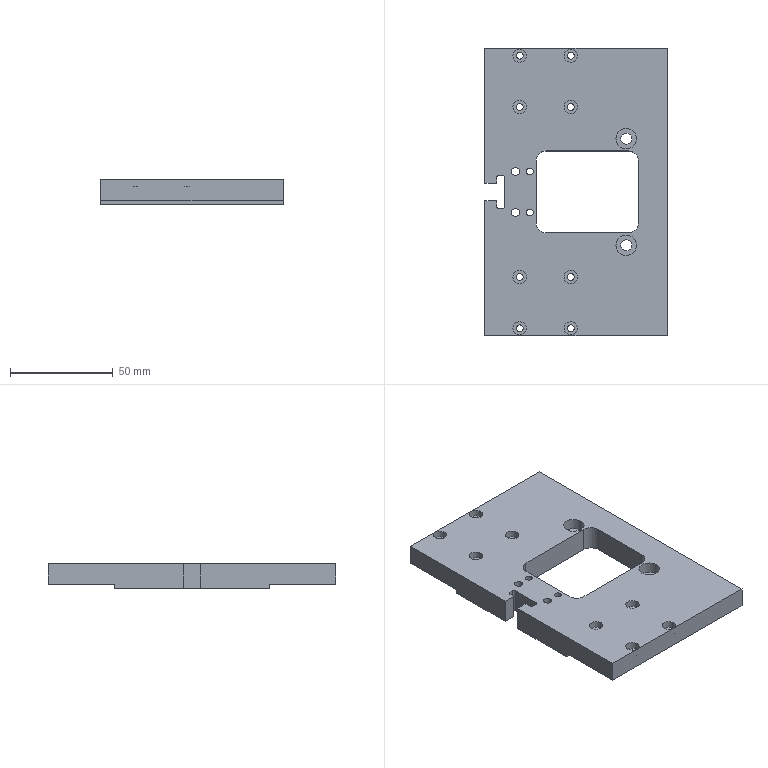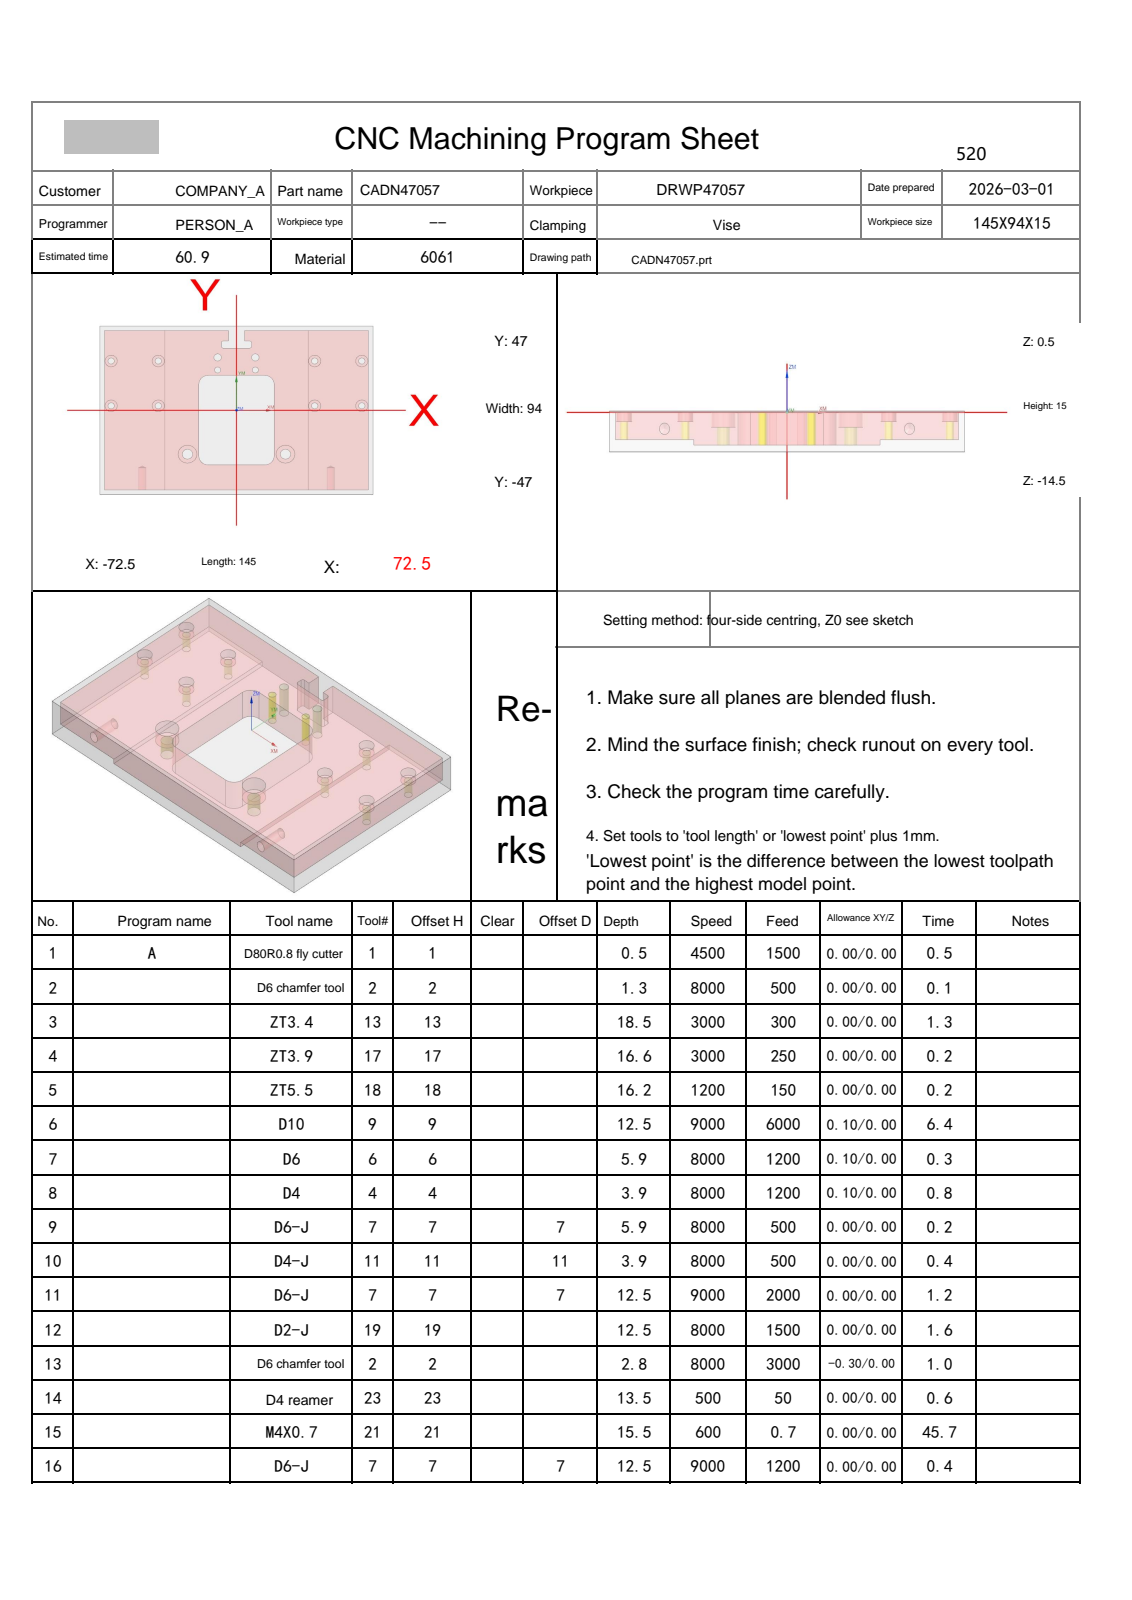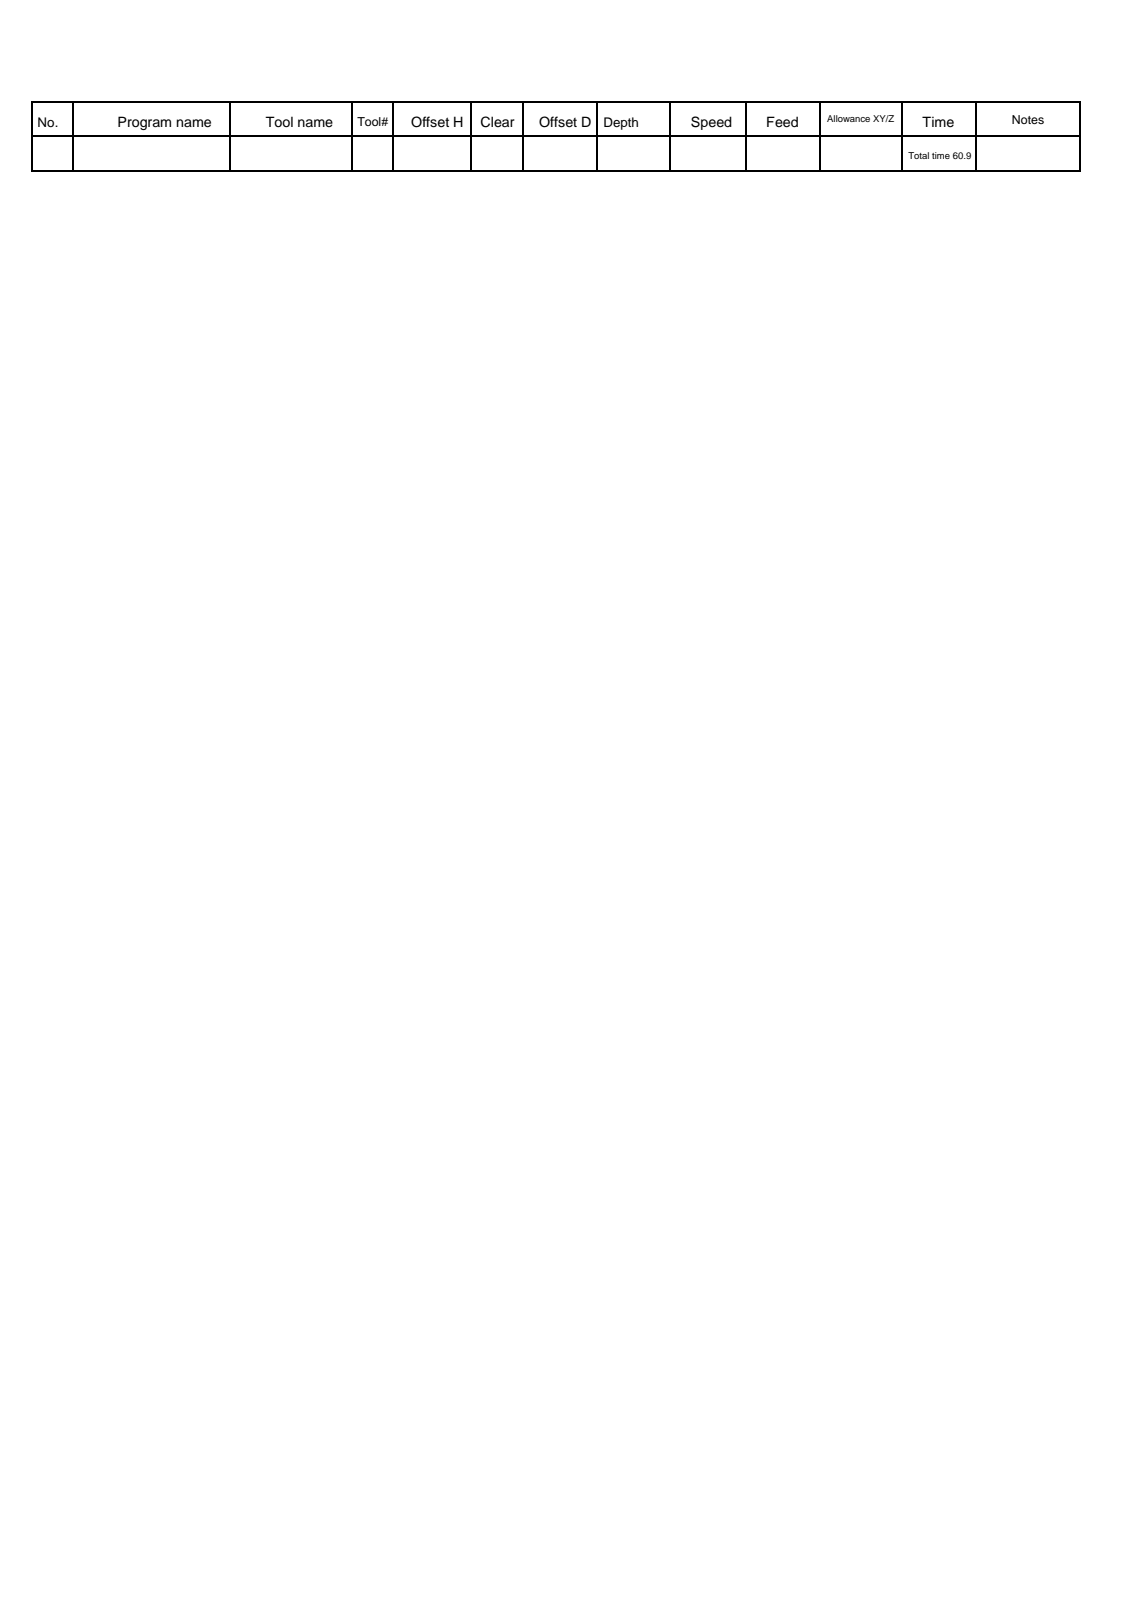NC program | NX | posted by the shop | part box 89 x 140 x 12 mm
Lines 949 to 2683 of 6684, first 1392 of 1735 lines:
N11 T07 M06
(D6-J  D=6. R=0. H=07 ce=0.00 di=0.00)
G00 G90 G54 X16.75 Y-5.7 M03 S9000
G43 H07 Z50.
M08
Z-5.45
G01 Z-5.95 F600.
G41 D07
X16.8
G03 X17. Y-5.5 I0.0 J.2
G01 Y14.5
G03 X15. Y16.5 I-2. J0.0
G01 X-15.
G03 X-17. Y14.5 I0.0 J-2.
G01 Y-25.5
G03 X-15. Y-27.5 I2. J0.0
G01 X15.
G03 X17. Y-25.5 I0.0 J2.
G01 Y-5.5
Y-5.
G03 X16.8 Y-4.8 I-.2 J0.0
G01 G40 X16.75
Z-5.45
G00 Z1.
Y-5.7
Z-11.4
G01 Z-11.9
G41 D07
X16.8
G03 X17. Y-5.5 I0.0 J.2
G01 Y14.5
G03 X15. Y16.5 I-2. J0.0
G01 X-15.
G03 X-17. Y14.5 I0.0 J-2.
G01 Y-25.5
G03 X-15. Y-27.5 I2. J0.0
G01 X15.
G03 X17. Y-25.5 I0.0 J2.
G01 Y-5.5
Y-5.
G03 X16.8 Y-4.8 I-.2 J0.0
G01 G40 X16.75
Z-11.4
G00 Z50.
G00 G90 X-2.228 Y47.539 M03 S8000
Z50.
Z.35
G01 X-2.232 Y47.532 Z.259 F2000.
X-2.243 Y47.513 Z.177
X-2.259 Y47.482 Z.103
X-2.278 Y47.441 Z.038
X-2.299 Y47.392 Z-.019
X-2.319 Y47.335 Z-.069
X-2.338 Y47.271 Z-.111
X-2.352 Y47.203 Z-.147
X-2.362 Y47.131 Z-.177
X-2.363 Y47.056 Z-.201
X-2.356 Y46.98 Z-.22
X-2.338 Y46.905 Z-.234
X-2.307 Y46.83 Z-.243
X-2.262 Y46.758 Z-.248
X-2.2 Y46.691 Z-.25
G02 X-1.25 Y44.5 I-2.05 J-2.191
G01 Y38.7
G02 X-1.422 Y37.7 I-3. J0.0
G01 X1.422
G02 X1.25 Y38.7 I2.828 J1.
G01 Y44.5
G02 X2.2 Y46.691 I3. J0.0
G01 X2.237 Y46.744 Z-.251
X2.24 Y46.801 Z-.252
X2.213 Y46.861 Z-.255
X2.157 Y46.923 Z-.259
X2.077 Y46.986 Z-.264
X1.974 Y47.049 Z-.27
X1.853 Y47.111 Z-.277
X1.715 Y47.172 Z-.284
X1.564 Y47.229 Z-.292
X1.402 Y47.283 Z-.3
X1.233 Y47.331 Z-.309
X1.059 Y47.375 Z-.318
X.635 Y47.452 Z-.34
X.206 Y47.49 Z-.363
X-.225 Y47.491 Z-.387
X-.653 Y47.453 Z-.41
X-1.075 Y47.376 Z-.432
X-1.262 Y47.329 Z-.442
X-1.444 Y47.275 Z-.452
X-1.616 Y47.215 Z-.46
X-1.775 Y47.151 Z-.469
X-1.917 Y47.084 Z-.476
X-2.038 Y47.016 Z-.483
X-2.134 Y46.947 Z-.489
X-2.202 Y46.878 Z-.494
X-2.238 Y46.812 Z-.497
X-2.239 Y46.749 Z-.499
X-2.2 Y46.691 Z-.5
G02 X-1.25 Y44.5 I-2.05 J-2.191
G01 Y38.7
G02 X-1.422 Y37.7 I-3. J0.0
G01 X1.422
G02 X1.25 Y38.7 I2.828 J1.
G01 Y44.5
G02 X2.2 Y46.691 I3. J0.0
G01 X2.237 Y46.744 Z-.501
X2.24 Y46.801 Z-.502
X2.213 Y46.861 Z-.505
X2.157 Y46.923 Z-.509
X2.077 Y46.986 Z-.514
X1.974 Y47.049 Z-.52
X1.853 Y47.111 Z-.527
X1.715 Y47.172 Z-.534
X1.564 Y47.229 Z-.542
X1.402 Y47.283 Z-.55
X1.233 Y47.331 Z-.559
X1.059 Y47.375 Z-.568
X.635 Y47.452 Z-.59
X.206 Y47.49 Z-.613
X-.225 Y47.491 Z-.637
X-.653 Y47.453 Z-.66
X-1.075 Y47.376 Z-.682
X-1.262 Y47.329 Z-.692
X-1.444 Y47.275 Z-.702
X-1.616 Y47.215 Z-.71
X-1.775 Y47.151 Z-.719
X-1.917 Y47.084 Z-.726
X-2.038 Y47.016 Z-.733
X-2.134 Y46.947 Z-.739
X-2.202 Y46.878 Z-.744
X-2.238 Y46.812 Z-.747
X-2.239 Y46.749 Z-.749
X-2.2 Y46.691 Z-.75
G02 X-1.25 Y44.5 I-2.05 J-2.191
G01 Y38.7
G02 X-1.422 Y37.7 I-3. J0.0
G01 X1.422
G02 X1.25 Y38.7 I2.828 J1.
G01 Y44.5
G02 X2.2 Y46.691 I3. J0.0
G01 X2.237 Y46.744 Z-.751
X2.24 Y46.801 Z-.752
X2.213 Y46.861 Z-.755
X2.157 Y46.923 Z-.759
X2.077 Y46.986 Z-.764
X1.974 Y47.049 Z-.77
X1.853 Y47.111 Z-.777
X1.715 Y47.172 Z-.784
X1.564 Y47.229 Z-.792
X1.402 Y47.283 Z-.8
X1.233 Y47.331 Z-.809
X1.059 Y47.375 Z-.818
X.635 Y47.452 Z-.84
X.206 Y47.49 Z-.863
X-.225 Y47.491 Z-.887
X-.653 Y47.453 Z-.91
X-1.075 Y47.376 Z-.932
X-1.262 Y47.329 Z-.942
X-1.444 Y47.275 Z-.952
X-1.616 Y47.215 Z-.96
X-1.775 Y47.151 Z-.969
X-1.917 Y47.084 Z-.976
X-2.038 Y47.016 Z-.983
X-2.134 Y46.947 Z-.989
X-2.202 Y46.878 Z-.994
X-2.238 Y46.812 Z-.997
X-2.239 Y46.749 Z-.999
X-2.2 Y46.691 Z-1.
G02 X-1.25 Y44.5 I-2.05 J-2.191
G01 Y38.7
G02 X-1.422 Y37.7 I-3. J0.0
G01 X1.422
G02 X1.25 Y38.7 I2.828 J1.
G01 Y44.5
G02 X2.2 Y46.691 I3. J0.0
G01 X2.237 Y46.744 Z-1.001
X2.24 Y46.801 Z-1.002
X2.213 Y46.861 Z-1.005
X2.157 Y46.923 Z-1.009
X2.077 Y46.986 Z-1.014
X1.974 Y47.049 Z-1.02
X1.853 Y47.111 Z-1.027
X1.715 Y47.172 Z-1.034
X1.564 Y47.229 Z-1.042
X1.402 Y47.283 Z-1.05
X1.233 Y47.331 Z-1.059
X1.059 Y47.375 Z-1.068
X.635 Y47.452 Z-1.09
X.206 Y47.49 Z-1.113
X-.225 Y47.491 Z-1.137
X-.653 Y47.453 Z-1.16
X-1.075 Y47.376 Z-1.182
X-1.262 Y47.329 Z-1.192
X-1.444 Y47.275 Z-1.202
X-1.616 Y47.215 Z-1.21
X-1.775 Y47.151 Z-1.219
X-1.917 Y47.084 Z-1.226
X-2.038 Y47.016 Z-1.233
X-2.134 Y46.947 Z-1.239
X-2.202 Y46.878 Z-1.244
X-2.238 Y46.812 Z-1.247
X-2.239 Y46.749 Z-1.249
X-2.2 Y46.691 Z-1.25
G02 X-1.25 Y44.5 I-2.05 J-2.191
G01 Y38.7
G02 X-1.422 Y37.7 I-3. J0.0
G01 X1.422
G02 X1.25 Y38.7 I2.828 J1.
G01 Y44.5
G02 X2.2 Y46.691 I3. J0.0
G01 X2.237 Y46.744 Z-1.251
X2.24 Y46.801 Z-1.252
X2.213 Y46.861 Z-1.255
X2.157 Y46.923 Z-1.259
X2.077 Y46.986 Z-1.264
X1.974 Y47.049 Z-1.27
X1.853 Y47.111 Z-1.277
X1.715 Y47.172 Z-1.284
X1.564 Y47.229 Z-1.292
X1.402 Y47.283 Z-1.3
X1.233 Y47.331 Z-1.309
X1.059 Y47.375 Z-1.318
X.635 Y47.452 Z-1.34
X.206 Y47.49 Z-1.363
X-.225 Y47.491 Z-1.387
X-.653 Y47.453 Z-1.41
X-1.075 Y47.376 Z-1.432
X-1.262 Y47.329 Z-1.442
X-1.444 Y47.275 Z-1.452
X-1.616 Y47.215 Z-1.46
X-1.775 Y47.151 Z-1.469
X-1.917 Y47.084 Z-1.476
X-2.038 Y47.016 Z-1.483
X-2.134 Y46.947 Z-1.489
X-2.202 Y46.878 Z-1.494
X-2.238 Y46.812 Z-1.497
X-2.239 Y46.749 Z-1.499
X-2.2 Y46.691 Z-1.5
G02 X-1.25 Y44.5 I-2.05 J-2.191
G01 Y38.7
G02 X-1.422 Y37.7 I-3. J0.0
G01 X1.422
G02 X1.25 Y38.7 I2.828 J1.
G01 Y44.5
G02 X2.2 Y46.691 I3. J0.0
G01 X2.237 Y46.744 Z-1.501
X2.24 Y46.801 Z-1.502
X2.213 Y46.861 Z-1.505
X2.157 Y46.923 Z-1.509
X2.077 Y46.986 Z-1.514
X1.974 Y47.049 Z-1.52
X1.853 Y47.111 Z-1.527
X1.715 Y47.172 Z-1.534
X1.564 Y47.229 Z-1.542
X1.402 Y47.283 Z-1.55
X1.233 Y47.331 Z-1.559
X1.059 Y47.375 Z-1.568
X.635 Y47.452 Z-1.59
X.206 Y47.49 Z-1.613
X-.225 Y47.491 Z-1.637
X-.653 Y47.453 Z-1.66
X-1.075 Y47.376 Z-1.682
X-1.262 Y47.329 Z-1.692
X-1.444 Y47.275 Z-1.702
X-1.616 Y47.215 Z-1.71
X-1.775 Y47.151 Z-1.719
X-1.917 Y47.084 Z-1.726
X-2.038 Y47.016 Z-1.733
X-2.134 Y46.947 Z-1.739
X-2.202 Y46.878 Z-1.744
X-2.238 Y46.812 Z-1.747
X-2.239 Y46.749 Z-1.749
X-2.2 Y46.691 Z-1.75
G02 X-1.25 Y44.5 I-2.05 J-2.191
G01 Y38.7
G02 X-1.422 Y37.7 I-3. J0.0
G01 X1.422
G02 X1.25 Y38.7 I2.828 J1.
G01 Y44.5
G02 X2.2 Y46.691 I3. J0.0
G01 X2.237 Y46.744 Z-1.751
X2.24 Y46.801 Z-1.752
X2.213 Y46.861 Z-1.755
X2.157 Y46.923 Z-1.759
X2.077 Y46.986 Z-1.764
X1.974 Y47.049 Z-1.77
X1.853 Y47.111 Z-1.777
X1.715 Y47.172 Z-1.784
X1.564 Y47.229 Z-1.792
X1.402 Y47.283 Z-1.8
X1.233 Y47.331 Z-1.809
X1.059 Y47.375 Z-1.818
X.635 Y47.452 Z-1.84
X.206 Y47.49 Z-1.863
X-.225 Y47.491 Z-1.887
X-.653 Y47.453 Z-1.91
X-1.075 Y47.376 Z-1.932
X-1.262 Y47.329 Z-1.942
X-1.444 Y47.275 Z-1.952
X-1.616 Y47.215 Z-1.96
X-1.775 Y47.151 Z-1.969
X-1.917 Y47.084 Z-1.976
X-2.038 Y47.016 Z-1.983
X-2.134 Y46.947 Z-1.989
X-2.202 Y46.878 Z-1.994
X-2.238 Y46.812 Z-1.997
X-2.239 Y46.749 Z-1.999
X-2.2 Y46.691 Z-2.
G02 X-1.25 Y44.5 I-2.05 J-2.191
G01 Y38.7
G02 X-1.422 Y37.7 I-3. J0.0
G01 X1.422
G02 X1.25 Y38.7 I2.828 J1.
G01 Y44.5
G02 X2.2 Y46.691 I3. J0.0
G01 X2.237 Y46.744 Z-2.001
X2.24 Y46.801 Z-2.002
X2.213 Y46.861 Z-2.005
X2.157 Y46.923 Z-2.009
X2.077 Y46.986 Z-2.014
X1.974 Y47.049 Z-2.02
X1.853 Y47.111 Z-2.027
X1.715 Y47.172 Z-2.034
X1.564 Y47.229 Z-2.042
X1.402 Y47.283 Z-2.05
X1.233 Y47.331 Z-2.059
X1.059 Y47.375 Z-2.068
X.635 Y47.452 Z-2.09
X.206 Y47.49 Z-2.113
X-.225 Y47.491 Z-2.137
X-.653 Y47.453 Z-2.16
X-1.075 Y47.376 Z-2.182
X-1.262 Y47.329 Z-2.192
X-1.444 Y47.275 Z-2.202
X-1.616 Y47.215 Z-2.21
X-1.775 Y47.151 Z-2.219
X-1.917 Y47.084 Z-2.226
X-2.038 Y47.016 Z-2.233
X-2.134 Y46.947 Z-2.239
X-2.202 Y46.878 Z-2.244
X-2.238 Y46.812 Z-2.247
X-2.239 Y46.749 Z-2.249
X-2.2 Y46.691 Z-2.25
G02 X-1.25 Y44.5 I-2.05 J-2.191
G01 Y38.7
G02 X-1.422 Y37.7 I-3. J0.0
G01 X1.422
G02 X1.25 Y38.7 I2.828 J1.
G01 Y44.5
G02 X2.2 Y46.691 I3. J0.0
G01 X2.237 Y46.744 Z-2.251
X2.24 Y46.801 Z-2.252
X2.213 Y46.861 Z-2.255
X2.157 Y46.923 Z-2.259
X2.077 Y46.986 Z-2.264
X1.974 Y47.049 Z-2.27
X1.853 Y47.111 Z-2.277
X1.715 Y47.172 Z-2.284
X1.564 Y47.229 Z-2.292
X1.402 Y47.283 Z-2.3
X1.233 Y47.331 Z-2.309
X1.059 Y47.375 Z-2.318
X.635 Y47.452 Z-2.34
X.206 Y47.49 Z-2.363
X-.225 Y47.491 Z-2.387
X-.653 Y47.453 Z-2.41
X-1.075 Y47.376 Z-2.432
X-1.262 Y47.329 Z-2.442
X-1.444 Y47.275 Z-2.452
X-1.616 Y47.215 Z-2.46
X-1.775 Y47.151 Z-2.469
X-1.917 Y47.084 Z-2.476
X-2.038 Y47.016 Z-2.483
X-2.134 Y46.947 Z-2.489
X-2.202 Y46.878 Z-2.494
X-2.238 Y46.812 Z-2.497
X-2.239 Y46.749 Z-2.499
X-2.2 Y46.691 Z-2.5
G02 X-1.25 Y44.5 I-2.05 J-2.191
G01 Y38.7
G02 X-1.422 Y37.7 I-3. J0.0
G01 X1.422
G02 X1.25 Y38.7 I2.828 J1.
G01 Y44.5
G02 X2.2 Y46.691 I3. J0.0
G01 X2.237 Y46.744 Z-2.501
X2.24 Y46.801 Z-2.502
X2.213 Y46.861 Z-2.505
X2.157 Y46.923 Z-2.509
X2.077 Y46.986 Z-2.514
X1.974 Y47.049 Z-2.52
X1.853 Y47.111 Z-2.527
X1.715 Y47.172 Z-2.534
X1.564 Y47.229 Z-2.542
X1.402 Y47.283 Z-2.55
X1.233 Y47.331 Z-2.559
X1.059 Y47.375 Z-2.568
X.635 Y47.452 Z-2.59
X.206 Y47.49 Z-2.613
X-.225 Y47.491 Z-2.637
X-.653 Y47.453 Z-2.66
X-1.075 Y47.376 Z-2.682
X-1.262 Y47.329 Z-2.692
X-1.444 Y47.275 Z-2.702
X-1.616 Y47.215 Z-2.71
X-1.775 Y47.151 Z-2.719
X-1.917 Y47.084 Z-2.726
X-2.038 Y47.016 Z-2.733
X-2.134 Y46.947 Z-2.739
X-2.202 Y46.878 Z-2.744
X-2.238 Y46.812 Z-2.747
X-2.239 Y46.749 Z-2.749
X-2.2 Y46.691 Z-2.75
G02 X-1.25 Y44.5 I-2.05 J-2.191
G01 Y38.7
G02 X-1.422 Y37.7 I-3. J0.0
G01 X1.422
G02 X1.25 Y38.7 I2.828 J1.
G01 Y44.5
G02 X2.2 Y46.691 I3. J0.0
G01 X2.237 Y46.744 Z-2.751
X2.24 Y46.801 Z-2.752
X2.213 Y46.861 Z-2.755
X2.157 Y46.923 Z-2.759
X2.077 Y46.986 Z-2.764
X1.974 Y47.049 Z-2.77
X1.853 Y47.111 Z-2.777
X1.715 Y47.172 Z-2.784
X1.564 Y47.229 Z-2.792
X1.402 Y47.283 Z-2.8
X1.233 Y47.331 Z-2.809
X1.059 Y47.375 Z-2.818
X.635 Y47.452 Z-2.84
X.206 Y47.49 Z-2.863
X-.225 Y47.491 Z-2.887
X-.653 Y47.453 Z-2.91
X-1.075 Y47.376 Z-2.932
X-1.262 Y47.329 Z-2.942
X-1.444 Y47.275 Z-2.952
X-1.616 Y47.215 Z-2.96
X-1.775 Y47.151 Z-2.969
X-1.917 Y47.084 Z-2.976
X-2.038 Y47.016 Z-2.983
X-2.134 Y46.947 Z-2.989
X-2.202 Y46.878 Z-2.994
X-2.238 Y46.812 Z-2.997
X-2.239 Y46.749 Z-2.999
X-2.2 Y46.691 Z-3.
G02 X-1.25 Y44.5 I-2.05 J-2.191
G01 Y38.7
G02 X-1.422 Y37.7 I-3. J0.0
G01 X1.422
G02 X1.25 Y38.7 I2.828 J1.
G01 Y44.5
G02 X2.2 Y46.691 I3. J0.0
G01 X2.237 Y46.744 Z-3.001
X2.24 Y46.801 Z-3.002
X2.213 Y46.861 Z-3.005
X2.157 Y46.923 Z-3.009
X2.077 Y46.986 Z-3.014
X1.974 Y47.049 Z-3.02
X1.853 Y47.111 Z-3.027
X1.715 Y47.172 Z-3.034
X1.564 Y47.229 Z-3.042
X1.402 Y47.283 Z-3.05
X1.233 Y47.331 Z-3.059
X1.059 Y47.375 Z-3.068
X.635 Y47.452 Z-3.09
X.206 Y47.49 Z-3.113
X-.225 Y47.491 Z-3.137
X-.653 Y47.453 Z-3.16
X-1.075 Y47.376 Z-3.182
X-1.262 Y47.329 Z-3.192
X-1.444 Y47.275 Z-3.202
X-1.616 Y47.215 Z-3.21
X-1.775 Y47.151 Z-3.219
X-1.917 Y47.084 Z-3.226
X-2.038 Y47.016 Z-3.233
X-2.134 Y46.947 Z-3.239
X-2.202 Y46.878 Z-3.244
X-2.238 Y46.812 Z-3.247
X-2.239 Y46.749 Z-3.249
X-2.2 Y46.691 Z-3.25
G02 X-1.25 Y44.5 I-2.05 J-2.191
G01 Y38.7
G02 X-1.422 Y37.7 I-3. J0.0
G01 X1.422
G02 X1.25 Y38.7 I2.828 J1.
G01 Y44.5
G02 X2.2 Y46.691 I3. J0.0
G01 X2.237 Y46.744 Z-3.251
X2.24 Y46.801 Z-3.252
X2.213 Y46.861 Z-3.255
X2.157 Y46.923 Z-3.259
X2.077 Y46.986 Z-3.264
X1.974 Y47.049 Z-3.27
X1.853 Y47.111 Z-3.277
X1.715 Y47.172 Z-3.284
X1.564 Y47.229 Z-3.292
X1.402 Y47.283 Z-3.3
X1.233 Y47.331 Z-3.309
X1.059 Y47.375 Z-3.318
X.635 Y47.452 Z-3.34
X.206 Y47.49 Z-3.363
X-.225 Y47.491 Z-3.387
X-.653 Y47.453 Z-3.41
X-1.075 Y47.376 Z-3.432
X-1.262 Y47.329 Z-3.442
X-1.444 Y47.275 Z-3.452
X-1.616 Y47.215 Z-3.46
X-1.775 Y47.151 Z-3.469
X-1.917 Y47.084 Z-3.476
X-2.038 Y47.016 Z-3.483
X-2.134 Y46.947 Z-3.489
X-2.202 Y46.878 Z-3.494
X-2.238 Y46.812 Z-3.497
X-2.239 Y46.749 Z-3.499
X-2.2 Y46.691 Z-3.5
G02 X-1.25 Y44.5 I-2.05 J-2.191
G01 Y38.7
G02 X-1.422 Y37.7 I-3. J0.0
G01 X1.422
G02 X1.25 Y38.7 I2.828 J1.
G01 Y44.5
G02 X2.2 Y46.691 I3. J0.0
G01 X2.237 Y46.744 Z-3.501
X2.24 Y46.801 Z-3.502
X2.213 Y46.861 Z-3.505
X2.157 Y46.923 Z-3.509
X2.077 Y46.986 Z-3.514
X1.974 Y47.049 Z-3.52
X1.853 Y47.111 Z-3.527
X1.715 Y47.172 Z-3.534
X1.564 Y47.229 Z-3.542
X1.402 Y47.283 Z-3.55
X1.233 Y47.331 Z-3.559
X1.059 Y47.375 Z-3.568
X.635 Y47.452 Z-3.59
X.206 Y47.49 Z-3.613
X-.225 Y47.491 Z-3.637
X-.653 Y47.453 Z-3.66
X-1.075 Y47.376 Z-3.682
X-1.262 Y47.329 Z-3.692
X-1.444 Y47.275 Z-3.702
X-1.616 Y47.215 Z-3.71
X-1.775 Y47.151 Z-3.719
X-1.917 Y47.084 Z-3.726
X-2.038 Y47.016 Z-3.733
X-2.134 Y46.947 Z-3.739
X-2.202 Y46.878 Z-3.744
X-2.238 Y46.812 Z-3.747
X-2.239 Y46.749 Z-3.749
X-2.2 Y46.691 Z-3.75
G02 X-1.25 Y44.5 I-2.05 J-2.191
G01 Y38.7
G02 X-1.422 Y37.7 I-3. J0.0
G01 X1.422
G02 X1.25 Y38.7 I2.828 J1.
G01 Y44.5
G02 X2.2 Y46.691 I3. J0.0
G01 X2.237 Y46.744 Z-3.751
X2.24 Y46.801 Z-3.752
X2.213 Y46.861 Z-3.755
X2.157 Y46.923 Z-3.759
X2.077 Y46.986 Z-3.764
X1.974 Y47.049 Z-3.77
X1.853 Y47.111 Z-3.777
X1.715 Y47.172 Z-3.784
X1.564 Y47.229 Z-3.792
X1.402 Y47.283 Z-3.8
X1.233 Y47.331 Z-3.809
X1.059 Y47.375 Z-3.818
X.635 Y47.452 Z-3.84
X.206 Y47.49 Z-3.863
X-.225 Y47.491 Z-3.887
X-.653 Y47.453 Z-3.91
X-1.075 Y47.376 Z-3.932
X-1.262 Y47.329 Z-3.942
X-1.444 Y47.275 Z-3.952
X-1.616 Y47.215 Z-3.96
X-1.775 Y47.151 Z-3.969
X-1.917 Y47.084 Z-3.976
X-2.038 Y47.016 Z-3.983
X-2.134 Y46.947 Z-3.989
X-2.202 Y46.878 Z-3.994
X-2.238 Y46.812 Z-3.997
X-2.239 Y46.749 Z-3.999
X-2.2 Y46.691 Z-4.
G02 X-1.25 Y44.5 I-2.05 J-2.191
G01 Y38.7
G02 X-1.422 Y37.7 I-3. J0.0
G01 X1.422
G02 X1.25 Y38.7 I2.828 J1.
G01 Y44.5
G02 X2.2 Y46.691 I3. J0.0
G01 X2.237 Y46.744 Z-4.001
X2.24 Y46.801 Z-4.002
X2.213 Y46.861 Z-4.005
X2.157 Y46.923 Z-4.009
X2.077 Y46.986 Z-4.014
X1.974 Y47.049 Z-4.02
X1.853 Y47.111 Z-4.027
X1.715 Y47.172 Z-4.034
X1.564 Y47.229 Z-4.042
X1.402 Y47.283 Z-4.05
X1.233 Y47.331 Z-4.059
X1.059 Y47.375 Z-4.068
X.635 Y47.452 Z-4.09
X.206 Y47.49 Z-4.113
X-.225 Y47.491 Z-4.137
X-.653 Y47.453 Z-4.16
X-1.075 Y47.376 Z-4.182
X-1.262 Y47.329 Z-4.192
X-1.444 Y47.275 Z-4.202
X-1.616 Y47.215 Z-4.21
X-1.775 Y47.151 Z-4.219
X-1.917 Y47.084 Z-4.226
X-2.038 Y47.016 Z-4.233
X-2.134 Y46.947 Z-4.239
X-2.202 Y46.878 Z-4.244
X-2.238 Y46.812 Z-4.247
X-2.239 Y46.749 Z-4.249
X-2.2 Y46.691 Z-4.25
G02 X-1.25 Y44.5 I-2.05 J-2.191
G01 Y38.7
G02 X-1.422 Y37.7 I-3. J0.0
G01 X1.422
G02 X1.25 Y38.7 I2.828 J1.
G01 Y44.5
G02 X2.2 Y46.691 I3. J0.0
G01 X2.237 Y46.744 Z-4.251
X2.24 Y46.801 Z-4.252
X2.213 Y46.861 Z-4.255
X2.157 Y46.923 Z-4.259
X2.077 Y46.986 Z-4.264
X1.974 Y47.049 Z-4.27
X1.853 Y47.111 Z-4.277
X1.715 Y47.172 Z-4.284
X1.564 Y47.229 Z-4.292
X1.402 Y47.283 Z-4.3
X1.233 Y47.331 Z-4.309
X1.059 Y47.375 Z-4.318
X.635 Y47.452 Z-4.34
X.206 Y47.49 Z-4.363
X-.225 Y47.491 Z-4.387
X-.653 Y47.453 Z-4.41
X-1.075 Y47.376 Z-4.432
X-1.262 Y47.329 Z-4.442
X-1.444 Y47.275 Z-4.452
X-1.616 Y47.215 Z-4.46
X-1.775 Y47.151 Z-4.469
X-1.917 Y47.084 Z-4.476
X-2.038 Y47.016 Z-4.483
X-2.134 Y46.947 Z-4.489
X-2.202 Y46.878 Z-4.494
X-2.238 Y46.812 Z-4.497
X-2.239 Y46.749 Z-4.499
X-2.2 Y46.691 Z-4.5
G02 X-1.25 Y44.5 I-2.05 J-2.191
G01 Y38.7
G02 X-1.422 Y37.7 I-3. J0.0
G01 X1.422
G02 X1.25 Y38.7 I2.828 J1.
G01 Y44.5
G02 X2.2 Y46.691 I3. J0.0
G01 X2.237 Y46.744 Z-4.501
X2.24 Y46.801 Z-4.502
X2.213 Y46.861 Z-4.505
X2.157 Y46.923 Z-4.509
X2.077 Y46.986 Z-4.514
X1.974 Y47.049 Z-4.52
X1.853 Y47.111 Z-4.527
X1.715 Y47.172 Z-4.534
X1.564 Y47.229 Z-4.542
X1.402 Y47.283 Z-4.55
X1.233 Y47.331 Z-4.559
X1.059 Y47.375 Z-4.568
X.635 Y47.452 Z-4.59
X.206 Y47.49 Z-4.613
X-.225 Y47.491 Z-4.637
X-.653 Y47.453 Z-4.66
X-1.075 Y47.376 Z-4.682
X-1.262 Y47.329 Z-4.692
X-1.444 Y47.275 Z-4.702
X-1.616 Y47.215 Z-4.71
X-1.775 Y47.151 Z-4.719
X-1.917 Y47.084 Z-4.726
X-2.038 Y47.016 Z-4.733
X-2.134 Y46.947 Z-4.739
X-2.202 Y46.878 Z-4.744
X-2.238 Y46.812 Z-4.747
X-2.239 Y46.749 Z-4.749
X-2.2 Y46.691 Z-4.75
G02 X-1.25 Y44.5 I-2.05 J-2.191
G01 Y38.7
G02 X-1.422 Y37.7 I-3. J0.0
G01 X1.422
G02 X1.25 Y38.7 I2.828 J1.
G01 Y44.5
G02 X2.2 Y46.691 I3. J0.0
G01 X2.237 Y46.744 Z-4.751
X2.24 Y46.801 Z-4.752
X2.213 Y46.861 Z-4.755
X2.157 Y46.923 Z-4.759
X2.077 Y46.986 Z-4.764
X1.974 Y47.049 Z-4.77
X1.853 Y47.111 Z-4.777
X1.715 Y47.172 Z-4.784
X1.564 Y47.229 Z-4.792
X1.402 Y47.283 Z-4.8
X1.233 Y47.331 Z-4.809
X1.059 Y47.375 Z-4.818
X.635 Y47.452 Z-4.84
X.206 Y47.49 Z-4.863
X-.225 Y47.491 Z-4.887
X-.653 Y47.453 Z-4.91
X-1.075 Y47.376 Z-4.932
X-1.262 Y47.329 Z-4.942
X-1.444 Y47.275 Z-4.952
X-1.616 Y47.215 Z-4.96
X-1.775 Y47.151 Z-4.969
X-1.917 Y47.084 Z-4.976
X-2.038 Y47.016 Z-4.983
X-2.134 Y46.947 Z-4.989
X-2.202 Y46.878 Z-4.994
X-2.238 Y46.812 Z-4.997
X-2.239 Y46.749 Z-4.999
X-2.2 Y46.691 Z-5.
G02 X-1.25 Y44.5 I-2.05 J-2.191
G01 Y38.7
G02 X-1.422 Y37.7 I-3. J0.0
G01 X1.422
G02 X1.25 Y38.7 I2.828 J1.
G01 Y44.5
G02 X2.2 Y46.691 I3. J0.0
G01 X2.237 Y46.744 Z-5.001
X2.24 Y46.801 Z-5.002
X2.213 Y46.861 Z-5.005
X2.157 Y46.923 Z-5.009
X2.077 Y46.986 Z-5.014
X1.974 Y47.049 Z-5.02
X1.853 Y47.111 Z-5.027
X1.715 Y47.172 Z-5.034
X1.564 Y47.229 Z-5.042
X1.402 Y47.283 Z-5.05
X1.233 Y47.331 Z-5.059
X1.059 Y47.375 Z-5.068
X.635 Y47.452 Z-5.09
X.206 Y47.49 Z-5.113
X-.225 Y47.491 Z-5.137
X-.653 Y47.453 Z-5.16
X-1.075 Y47.376 Z-5.182
X-1.262 Y47.329 Z-5.192
X-1.444 Y47.275 Z-5.202
X-1.616 Y47.215 Z-5.21
X-1.775 Y47.151 Z-5.219
X-1.917 Y47.084 Z-5.226
X-2.038 Y47.016 Z-5.233
X-2.134 Y46.947 Z-5.239
X-2.202 Y46.878 Z-5.244
X-2.238 Y46.812 Z-5.247
X-2.239 Y46.749 Z-5.249
X-2.2 Y46.691 Z-5.25
G02 X-1.25 Y44.5 I-2.05 J-2.191
G01 Y38.7
G02 X-1.422 Y37.7 I-3. J0.0
G01 X1.422
G02 X1.25 Y38.7 I2.828 J1.
G01 Y44.5
G02 X2.2 Y46.691 I3. J0.0
G01 X2.237 Y46.744 Z-5.251
X2.24 Y46.801 Z-5.252
X2.213 Y46.861 Z-5.255
X2.157 Y46.923 Z-5.259
X2.077 Y46.986 Z-5.264
X1.974 Y47.049 Z-5.27
X1.853 Y47.111 Z-5.277
X1.715 Y47.172 Z-5.284
X1.564 Y47.229 Z-5.292
X1.402 Y47.283 Z-5.3
X1.233 Y47.331 Z-5.309
X1.059 Y47.375 Z-5.318
X.635 Y47.452 Z-5.34
X.206 Y47.49 Z-5.363
X-.225 Y47.491 Z-5.387
X-.653 Y47.453 Z-5.41
X-1.075 Y47.376 Z-5.432
X-1.262 Y47.329 Z-5.442
X-1.444 Y47.275 Z-5.452
X-1.616 Y47.215 Z-5.46
X-1.775 Y47.151 Z-5.469
X-1.917 Y47.084 Z-5.476
X-2.038 Y47.016 Z-5.483
X-2.134 Y46.947 Z-5.489
X-2.202 Y46.878 Z-5.494
X-2.238 Y46.812 Z-5.497
X-2.239 Y46.749 Z-5.499
X-2.2 Y46.691 Z-5.5
G02 X-1.25 Y44.5 I-2.05 J-2.191
G01 Y38.7
G02 X-1.422 Y37.7 I-3. J0.0
G01 X1.422
G02 X1.25 Y38.7 I2.828 J1.
G01 Y44.5
G02 X2.2 Y46.691 I3. J0.0
G01 X2.237 Y46.744 Z-5.501
X2.24 Y46.801 Z-5.502
X2.213 Y46.861 Z-5.505
X2.157 Y46.923 Z-5.509
X2.077 Y46.986 Z-5.514
X1.974 Y47.049 Z-5.52
X1.853 Y47.111 Z-5.527
X1.715 Y47.172 Z-5.534
X1.564 Y47.229 Z-5.542
X1.402 Y47.283 Z-5.55
X1.233 Y47.331 Z-5.559
X1.059 Y47.375 Z-5.568
X.635 Y47.452 Z-5.59
X.206 Y47.49 Z-5.613
X-.225 Y47.491 Z-5.637
X-.653 Y47.453 Z-5.66
X-1.075 Y47.376 Z-5.682
X-1.262 Y47.329 Z-5.692
X-1.444 Y47.275 Z-5.702
X-1.616 Y47.215 Z-5.71
X-1.775 Y47.151 Z-5.719
X-1.917 Y47.084 Z-5.726
X-2.038 Y47.016 Z-5.733
X-2.134 Y46.947 Z-5.739
X-2.202 Y46.878 Z-5.744
X-2.238 Y46.812 Z-5.747
X-2.239 Y46.749 Z-5.749
X-2.2 Y46.691 Z-5.75
G02 X-1.25 Y44.5 I-2.05 J-2.191
G01 Y38.7
G02 X-1.422 Y37.7 I-3. J0.0
G01 X1.422
G02 X1.25 Y38.7 I2.828 J1.
G01 Y44.5
G02 X2.2 Y46.691 I3. J0.0
G01 X2.237 Y46.744 Z-5.751
X2.24 Y46.801 Z-5.752
X2.213 Y46.861 Z-5.755
X2.157 Y46.923 Z-5.759
X2.077 Y46.986 Z-5.764
X1.974 Y47.049 Z-5.77
X1.853 Y47.111 Z-5.777
X1.715 Y47.172 Z-5.784
X1.564 Y47.229 Z-5.792
X1.402 Y47.283 Z-5.8
X1.233 Y47.331 Z-5.809
X1.059 Y47.375 Z-5.818
X.635 Y47.452 Z-5.84
X.206 Y47.49 Z-5.863
X-.225 Y47.491 Z-5.887
X-.653 Y47.453 Z-5.91
X-1.075 Y47.376 Z-5.932
X-1.262 Y47.329 Z-5.942
X-1.444 Y47.275 Z-5.952
X-1.616 Y47.215 Z-5.96
X-1.775 Y47.151 Z-5.969
X-1.917 Y47.084 Z-5.976
X-2.038 Y47.016 Z-5.983
X-2.134 Y46.947 Z-5.989
X-2.202 Y46.878 Z-5.994
X-2.238 Y46.812 Z-5.997
X-2.239 Y46.749 Z-5.999
X-2.2 Y46.691 Z-6.
G02 X-1.25 Y44.5 I-2.05 J-2.191
G01 Y38.7
G02 X-1.422 Y37.7 I-3. J0.0
G01 X1.422
G02 X1.25 Y38.7 I2.828 J1.
G01 Y44.5
G02 X2.2 Y46.691 I3. J0.0
G01 X2.237 Y46.744 Z-6.001
X2.24 Y46.801 Z-6.002
X2.213 Y46.861 Z-6.005
X2.157 Y46.923 Z-6.009
X2.077 Y46.986 Z-6.014
X1.974 Y47.049 Z-6.02
X1.853 Y47.111 Z-6.027
X1.715 Y47.172 Z-6.034
X1.564 Y47.229 Z-6.042
X1.402 Y47.283 Z-6.05
X1.233 Y47.331 Z-6.059
X1.059 Y47.375 Z-6.068
X.635 Y47.452 Z-6.09
X.206 Y47.49 Z-6.113
X-.225 Y47.491 Z-6.137
X-.653 Y47.453 Z-6.16
X-1.075 Y47.376 Z-6.182
X-1.262 Y47.329 Z-6.192
X-1.444 Y47.275 Z-6.202
X-1.616 Y47.215 Z-6.21
X-1.775 Y47.151 Z-6.219
X-1.917 Y47.084 Z-6.226
X-2.038 Y47.016 Z-6.233
X-2.134 Y46.947 Z-6.239
X-2.202 Y46.878 Z-6.244
X-2.238 Y46.812 Z-6.247
X-2.239 Y46.749 Z-6.249
X-2.2 Y46.691 Z-6.25
G02 X-1.25 Y44.5 I-2.05 J-2.191
G01 Y38.7
G02 X-1.422 Y37.7 I-3. J0.0
G01 X1.422
G02 X1.25 Y38.7 I2.828 J1.
G01 Y44.5
G02 X2.2 Y46.691 I3. J0.0
G01 X2.237 Y46.744 Z-6.251
X2.24 Y46.801 Z-6.252
X2.213 Y46.861 Z-6.255
X2.157 Y46.923 Z-6.259
X2.077 Y46.986 Z-6.264
X1.974 Y47.049 Z-6.27
X1.853 Y47.111 Z-6.277
X1.715 Y47.172 Z-6.284
X1.564 Y47.229 Z-6.292
X1.402 Y47.283 Z-6.3
X1.233 Y47.331 Z-6.309
X1.059 Y47.375 Z-6.318
X.635 Y47.452 Z-6.34
X.206 Y47.49 Z-6.363
X-.225 Y47.491 Z-6.387
X-.653 Y47.453 Z-6.41
X-1.075 Y47.376 Z-6.432
X-1.262 Y47.329 Z-6.442
X-1.444 Y47.275 Z-6.452
X-1.616 Y47.215 Z-6.46
X-1.775 Y47.151 Z-6.469
X-1.917 Y47.084 Z-6.476
X-2.038 Y47.016 Z-6.483
X-2.134 Y46.947 Z-6.489
X-2.202 Y46.878 Z-6.494
X-2.238 Y46.812 Z-6.497
X-2.239 Y46.749 Z-6.499
X-2.2 Y46.691 Z-6.5
G02 X-1.25 Y44.5 I-2.05 J-2.191
G01 Y38.7
G02 X-1.422 Y37.7 I-3. J0.0
G01 X1.422
G02 X1.25 Y38.7 I2.828 J1.
G01 Y44.5
G02 X2.2 Y46.691 I3. J0.0
G01 X2.237 Y46.744 Z-6.501
X2.24 Y46.801 Z-6.502
X2.213 Y46.861 Z-6.505
X2.157 Y46.923 Z-6.509
X2.077 Y46.986 Z-6.514
X1.974 Y47.049 Z-6.52
X1.853 Y47.111 Z-6.527
X1.715 Y47.172 Z-6.534
X1.564 Y47.229 Z-6.542
X1.402 Y47.283 Z-6.55
X1.233 Y47.331 Z-6.559
X1.059 Y47.375 Z-6.568
X.635 Y47.452 Z-6.59
X.206 Y47.49 Z-6.613
X-.225 Y47.491 Z-6.637
X-.653 Y47.453 Z-6.66
X-1.075 Y47.376 Z-6.682
X-1.262 Y47.329 Z-6.692
X-1.444 Y47.275 Z-6.702
X-1.616 Y47.215 Z-6.71
X-1.775 Y47.151 Z-6.719
X-1.917 Y47.084 Z-6.726
X-2.038 Y47.016 Z-6.733
X-2.134 Y46.947 Z-6.739
X-2.202 Y46.878 Z-6.744
X-2.238 Y46.812 Z-6.747
X-2.239 Y46.749 Z-6.749
X-2.2 Y46.691 Z-6.75
G02 X-1.25 Y44.5 I-2.05 J-2.191
G01 Y38.7
G02 X-1.422 Y37.7 I-3. J0.0
G01 X1.422
G02 X1.25 Y38.7 I2.828 J1.
G01 Y44.5
G02 X2.2 Y46.691 I3. J0.0
G01 X2.237 Y46.744 Z-6.751
X2.24 Y46.801 Z-6.752
X2.213 Y46.861 Z-6.755
X2.157 Y46.923 Z-6.759
X2.077 Y46.986 Z-6.764
X1.974 Y47.049 Z-6.77
X1.853 Y47.111 Z-6.777
X1.715 Y47.172 Z-6.784
X1.564 Y47.229 Z-6.792
X1.402 Y47.283 Z-6.8
X1.233 Y47.331 Z-6.809
X1.059 Y47.375 Z-6.818
X.635 Y47.452 Z-6.84
X.206 Y47.49 Z-6.863
X-.225 Y47.491 Z-6.887
X-.653 Y47.453 Z-6.91
X-1.075 Y47.376 Z-6.932
X-1.262 Y47.329 Z-6.942
X-1.444 Y47.275 Z-6.952
X-1.616 Y47.215 Z-6.96
X-1.775 Y47.151 Z-6.969
X-1.917 Y47.084 Z-6.976
X-2.038 Y47.016 Z-6.983
X-2.134 Y46.947 Z-6.989
X-2.202 Y46.878 Z-6.994
X-2.238 Y46.812 Z-6.997
X-2.239 Y46.749 Z-6.999
X-2.2 Y46.691 Z-7.
G02 X-1.25 Y44.5 I-2.05 J-2.191
G01 Y38.7
G02 X-1.422 Y37.7 I-3. J0.0
G01 X1.422
G02 X1.25 Y38.7 I2.828 J1.
G01 Y44.5
G02 X2.2 Y46.691 I3. J0.0
G01 X2.237 Y46.744 Z-7.001
X2.24 Y46.801 Z-7.002
X2.213 Y46.861 Z-7.005
X2.157 Y46.923 Z-7.009
X2.077 Y46.986 Z-7.014
X1.974 Y47.049 Z-7.02
X1.853 Y47.111 Z-7.027
X1.715 Y47.172 Z-7.034
X1.564 Y47.229 Z-7.042
X1.402 Y47.283 Z-7.05
X1.233 Y47.331 Z-7.059
X1.059 Y47.375 Z-7.068
X.635 Y47.452 Z-7.09
X.206 Y47.49 Z-7.113
X-.225 Y47.491 Z-7.137
X-.653 Y47.453 Z-7.16
X-1.075 Y47.376 Z-7.182
X-1.262 Y47.329 Z-7.192
X-1.444 Y47.275 Z-7.202
X-1.616 Y47.215 Z-7.21
X-1.775 Y47.151 Z-7.219
X-1.917 Y47.084 Z-7.226
X-2.038 Y47.016 Z-7.233
X-2.134 Y46.947 Z-7.239
X-2.202 Y46.878 Z-7.244
X-2.238 Y46.812 Z-7.247
X-2.239 Y46.749 Z-7.249
X-2.2 Y46.691 Z-7.25
G02 X-1.25 Y44.5 I-2.05 J-2.191
G01 Y38.7
G02 X-1.422 Y37.7 I-3. J0.0
G01 X1.422
G02 X1.25 Y38.7 I2.828 J1.
G01 Y44.5
G02 X2.2 Y46.691 I3. J0.0
G01 X2.237 Y46.744 Z-7.251
X2.24 Y46.801 Z-7.252
X2.213 Y46.861 Z-7.255
X2.157 Y46.923 Z-7.259
X2.077 Y46.986 Z-7.264
X1.974 Y47.049 Z-7.27
X1.853 Y47.111 Z-7.277
X1.715 Y47.172 Z-7.284
X1.564 Y47.229 Z-7.292
X1.402 Y47.283 Z-7.3
X1.233 Y47.331 Z-7.309
X1.059 Y47.375 Z-7.318
X.635 Y47.452 Z-7.34
X.206 Y47.49 Z-7.363
X-.225 Y47.491 Z-7.387
X-.653 Y47.453 Z-7.41
X-1.075 Y47.376 Z-7.432
X-1.262 Y47.329 Z-7.442
X-1.444 Y47.275 Z-7.452
X-1.616 Y47.215 Z-7.46
X-1.775 Y47.151 Z-7.469
X-1.917 Y47.084 Z-7.476
X-2.038 Y47.016 Z-7.483
X-2.134 Y46.947 Z-7.489
X-2.202 Y46.878 Z-7.494
X-2.238 Y46.812 Z-7.497
X-2.239 Y46.749 Z-7.499
X-2.2 Y46.691 Z-7.5
G02 X-1.25 Y44.5 I-2.05 J-2.191
G01 Y38.7
G02 X-1.422 Y37.7 I-3. J0.0
G01 X1.422
G02 X1.25 Y38.7 I2.828 J1.
G01 Y44.5
G02 X2.2 Y46.691 I3. J0.0
G01 X2.237 Y46.744 Z-7.501
X2.24 Y46.801 Z-7.502
X2.213 Y46.861 Z-7.505
X2.157 Y46.923 Z-7.509
X2.077 Y46.986 Z-7.514
X1.974 Y47.049 Z-7.52
X1.853 Y47.111 Z-7.527
X1.715 Y47.172 Z-7.534
X1.564 Y47.229 Z-7.542
X1.402 Y47.283 Z-7.55
X1.233 Y47.331 Z-7.559
X1.059 Y47.375 Z-7.568
X.635 Y47.452 Z-7.59
X.206 Y47.49 Z-7.613
X-.225 Y47.491 Z-7.637
X-.653 Y47.453 Z-7.66
X-1.075 Y47.376 Z-7.682
X-1.262 Y47.329 Z-7.692
X-1.444 Y47.275 Z-7.702
X-1.616 Y47.215 Z-7.71
X-1.775 Y47.151 Z-7.719
X-1.917 Y47.084 Z-7.726
X-2.038 Y47.016 Z-7.733
X-2.134 Y46.947 Z-7.739
X-2.202 Y46.878 Z-7.744
X-2.238 Y46.812 Z-7.747
X-2.239 Y46.749 Z-7.749
X-2.2 Y46.691 Z-7.75
G02 X-1.25 Y44.5 I-2.05 J-2.191
G01 Y38.7
G02 X-1.422 Y37.7 I-3. J0.0
G01 X1.422
G02 X1.25 Y38.7 I2.828 J1.
G01 Y44.5
G02 X2.2 Y46.691 I3. J0.0
G01 X2.237 Y46.744 Z-7.751
X2.24 Y46.801 Z-7.752
X2.213 Y46.861 Z-7.755
X2.157 Y46.923 Z-7.759
X2.077 Y46.986 Z-7.764
X1.974 Y47.049 Z-7.77
X1.853 Y47.111 Z-7.777
X1.715 Y47.172 Z-7.784
X1.564 Y47.229 Z-7.792
X1.402 Y47.283 Z-7.8
X1.233 Y47.331 Z-7.809
X1.059 Y47.375 Z-7.818
X.635 Y47.452 Z-7.84
X.206 Y47.49 Z-7.863
X-.225 Y47.491 Z-7.887
X-.653 Y47.453 Z-7.91
X-1.075 Y47.376 Z-7.932
X-1.262 Y47.329 Z-7.942
X-1.444 Y47.275 Z-7.952
X-1.616 Y47.215 Z-7.96
X-1.775 Y47.151 Z-7.969
X-1.917 Y47.084 Z-7.976
X-2.038 Y47.016 Z-7.983
X-2.134 Y46.947 Z-7.989
X-2.202 Y46.878 Z-7.994
X-2.238 Y46.812 Z-7.997
X-2.239 Y46.749 Z-7.999
X-2.2 Y46.691 Z-8.
G02 X-1.25 Y44.5 I-2.05 J-2.191
G01 Y38.7
G02 X-1.422 Y37.7 I-3. J0.0
G01 X1.422
G02 X1.25 Y38.7 I2.828 J1.
G01 Y44.5
G02 X2.2 Y46.691 I3. J0.0
G01 X2.237 Y46.744 Z-8.001
X2.24 Y46.801 Z-8.002
X2.213 Y46.861 Z-8.005
X2.157 Y46.923 Z-8.009
X2.077 Y46.986 Z-8.014
X1.974 Y47.049 Z-8.02
X1.853 Y47.111 Z-8.027
X1.715 Y47.172 Z-8.034
X1.564 Y47.229 Z-8.042
X1.402 Y47.283 Z-8.05
X1.233 Y47.331 Z-8.059
X1.059 Y47.375 Z-8.068
X.635 Y47.452 Z-8.09
X.206 Y47.49 Z-8.113
X-.225 Y47.491 Z-8.137
X-.653 Y47.453 Z-8.16
X-1.075 Y47.376 Z-8.182
X-1.262 Y47.329 Z-8.192
X-1.444 Y47.275 Z-8.202
X-1.616 Y47.215 Z-8.21
X-1.775 Y47.151 Z-8.219
X-1.917 Y47.084 Z-8.226
X-2.038 Y47.016 Z-8.233
X-2.134 Y46.947 Z-8.239
X-2.202 Y46.878 Z-8.244
X-2.238 Y46.812 Z-8.247
X-2.239 Y46.749 Z-8.249
X-2.2 Y46.691 Z-8.25
G02 X-1.25 Y44.5 I-2.05 J-2.191
G01 Y38.7
G02 X-1.422 Y37.7 I-3. J0.0
G01 X1.422
G02 X1.25 Y38.7 I2.828 J1.
G01 Y44.5
G02 X2.2 Y46.691 I3. J0.0
G01 X2.237 Y46.744 Z-8.251
X2.24 Y46.801 Z-8.252
X2.213 Y46.861 Z-8.255
X2.157 Y46.923 Z-8.259
X2.077 Y46.986 Z-8.264
X1.974 Y47.049 Z-8.27
X1.853 Y47.111 Z-8.277
X1.715 Y47.172 Z-8.284
X1.564 Y47.229 Z-8.292
X1.402 Y47.283 Z-8.3
X1.233 Y47.331 Z-8.309
X1.059 Y47.375 Z-8.318
X.635 Y47.452 Z-8.34
X.206 Y47.49 Z-8.363
X-.225 Y47.491 Z-8.387
X-.653 Y47.453 Z-8.41
X-1.075 Y47.376 Z-8.432
X-1.262 Y47.329 Z-8.442
X-1.444 Y47.275 Z-8.452
X-1.616 Y47.215 Z-8.46
X-1.775 Y47.151 Z-8.469
X-1.917 Y47.084 Z-8.476
X-2.038 Y47.016 Z-8.483
X-2.134 Y46.947 Z-8.489
X-2.202 Y46.878 Z-8.494
X-2.238 Y46.812 Z-8.497
X-2.239 Y46.749 Z-8.499
X-2.2 Y46.691 Z-8.5
G02 X-1.25 Y44.5 I-2.05 J-2.191
G01 Y38.7
G02 X-1.422 Y37.7 I-3. J0.0
G01 X1.422
G02 X1.25 Y38.7 I2.828 J1.
G01 Y44.5
G02 X2.2 Y46.691 I3. J0.0
G01 X2.237 Y46.744 Z-8.501
X2.24 Y46.801 Z-8.502
X2.213 Y46.861 Z-8.505
X2.157 Y46.923 Z-8.509
X2.077 Y46.986 Z-8.514
X1.974 Y47.049 Z-8.52
X1.853 Y47.111 Z-8.527
X1.715 Y47.172 Z-8.534
X1.564 Y47.229 Z-8.542
X1.402 Y47.283 Z-8.55
X1.233 Y47.331 Z-8.559
X1.059 Y47.375 Z-8.568
X.635 Y47.452 Z-8.59
X.206 Y47.49 Z-8.613
X-.225 Y47.491 Z-8.637
X-.653 Y47.453 Z-8.66
X-1.075 Y47.376 Z-8.682
X-1.262 Y47.329 Z-8.692
X-1.444 Y47.275 Z-8.702
X-1.616 Y47.215 Z-8.71
X-1.775 Y47.151 Z-8.719
X-1.917 Y47.084 Z-8.726
X-2.038 Y47.016 Z-8.733
X-2.134 Y46.947 Z-8.739
X-2.202 Y46.878 Z-8.744
X-2.238 Y46.812 Z-8.747
X-2.239 Y46.749 Z-8.749
X-2.2 Y46.691 Z-8.75
G02 X-1.25 Y44.5 I-2.05 J-2.191
G01 Y38.7
G02 X-1.422 Y37.7 I-3. J0.0
G01 X1.422
G02 X1.25 Y38.7 I2.828 J1.
G01 Y44.5
G02 X2.2 Y46.691 I3. J0.0
G01 X2.237 Y46.744 Z-8.751
X2.24 Y46.801 Z-8.752
X2.213 Y46.861 Z-8.755
X2.157 Y46.923 Z-8.759
X2.077 Y46.986 Z-8.764
X1.974 Y47.049 Z-8.77
X1.853 Y47.111 Z-8.777
X1.715 Y47.172 Z-8.784
X1.564 Y47.229 Z-8.792
X1.402 Y47.283 Z-8.8
X1.233 Y47.331 Z-8.809
X1.059 Y47.375 Z-8.818
X.635 Y47.452 Z-8.84
X.206 Y47.49 Z-8.863
X-.225 Y47.491 Z-8.887
X-.653 Y47.453 Z-8.91
X-1.075 Y47.376 Z-8.932
X-1.262 Y47.329 Z-8.942
X-1.444 Y47.275 Z-8.952
X-1.616 Y47.215 Z-8.96
X-1.775 Y47.151 Z-8.969
X-1.917 Y47.084 Z-8.976
X-2.038 Y47.016 Z-8.983
X-2.134 Y46.947 Z-8.989
X-2.202 Y46.878 Z-8.994
X-2.238 Y46.812 Z-8.997
X-2.239 Y46.749 Z-8.999
X-2.2 Y46.691 Z-9.
G02 X-1.25 Y44.5 I-2.05 J-2.191
G01 Y38.7
G02 X-1.422 Y37.7 I-3. J0.0
G01 X1.422
G02 X1.25 Y38.7 I2.828 J1.
G01 Y44.5
G02 X2.2 Y46.691 I3. J0.0
G01 X2.237 Y46.744 Z-9.001
X2.24 Y46.801 Z-9.002
X2.213 Y46.861 Z-9.005
X2.157 Y46.923 Z-9.009
X2.077 Y46.986 Z-9.014
X1.974 Y47.049 Z-9.02
X1.853 Y47.111 Z-9.027
X1.715 Y47.172 Z-9.034
X1.564 Y47.229 Z-9.042
X1.402 Y47.283 Z-9.05
X1.233 Y47.331 Z-9.059
X1.059 Y47.375 Z-9.068
X.635 Y47.452 Z-9.09
X.206 Y47.49 Z-9.113
X-.225 Y47.491 Z-9.137
X-.653 Y47.453 Z-9.16
X-1.075 Y47.376 Z-9.182
X-1.262 Y47.329 Z-9.192
X-1.444 Y47.275 Z-9.202
X-1.616 Y47.215 Z-9.21
X-1.775 Y47.151 Z-9.219
X-1.917 Y47.084 Z-9.226
X-2.038 Y47.016 Z-9.233
X-2.134 Y46.947 Z-9.239
X-2.202 Y46.878 Z-9.244
X-2.238 Y46.812 Z-9.247
X-2.239 Y46.749 Z-9.249
X-2.2 Y46.691 Z-9.25
G02 X-1.25 Y44.5 I-2.05 J-2.191
G01 Y38.7
G02 X-1.422 Y37.7 I-3. J0.0
G01 X1.422
G02 X1.25 Y38.7 I2.828 J1.
G01 Y44.5
G02 X2.2 Y46.691 I3. J0.0
G01 X2.237 Y46.744 Z-9.251
X2.24 Y46.801 Z-9.252
X2.213 Y46.861 Z-9.255
X2.157 Y46.923 Z-9.259
X2.077 Y46.986 Z-9.264
X1.974 Y47.049 Z-9.27
X1.853 Y47.111 Z-9.277
X1.715 Y47.172 Z-9.284
X1.564 Y47.229 Z-9.292
X1.402 Y47.283 Z-9.3
X1.233 Y47.331 Z-9.309
X1.059 Y47.375 Z-9.318
X.635 Y47.452 Z-9.34
X.206 Y47.49 Z-9.363
X-.225 Y47.491 Z-9.387
X-.653 Y47.453 Z-9.41
X-1.075 Y47.376 Z-9.432
X-1.262 Y47.329 Z-9.442
X-1.444 Y47.275 Z-9.452
X-1.616 Y47.215 Z-9.46
X-1.775 Y47.151 Z-9.469
X-1.917 Y47.084 Z-9.476
X-2.038 Y47.016 Z-9.483
X-2.134 Y46.947 Z-9.489
X-2.202 Y46.878 Z-9.494
X-2.238 Y46.812 Z-9.497
X-2.239 Y46.749 Z-9.499
X-2.2 Y46.691 Z-9.5
G02 X-1.25 Y44.5 I-2.05 J-2.191
G01 Y38.7
G02 X-1.422 Y37.7 I-3. J0.0
G01 X1.422
G02 X1.25 Y38.7 I2.828 J1.
G01 Y44.5
G02 X2.2 Y46.691 I3. J0.0
G01 X2.237 Y46.744 Z-9.501
X2.24 Y46.801 Z-9.502
X2.213 Y46.861 Z-9.505
X2.157 Y46.923 Z-9.509
X2.077 Y46.986 Z-9.514
X1.974 Y47.049 Z-9.52
X1.853 Y47.111 Z-9.527
X1.715 Y47.172 Z-9.534
X1.564 Y47.229 Z-9.542
X1.402 Y47.283 Z-9.55
X1.233 Y47.331 Z-9.559
X1.059 Y47.375 Z-9.568
X.635 Y47.452 Z-9.59
X.206 Y47.49 Z-9.613
X-.225 Y47.491 Z-9.637
X-.653 Y47.453 Z-9.66
X-1.075 Y47.376 Z-9.682
X-1.262 Y47.329 Z-9.692
X-1.444 Y47.275 Z-9.702
X-1.616 Y47.215 Z-9.71
X-1.775 Y47.151 Z-9.719
X-1.917 Y47.084 Z-9.726
X-2.038 Y47.016 Z-9.733
X-2.134 Y46.947 Z-9.739
X-2.202 Y46.878 Z-9.744
X-2.238 Y46.812 Z-9.747
X-2.239 Y46.749 Z-9.749
X-2.2 Y46.691 Z-9.75